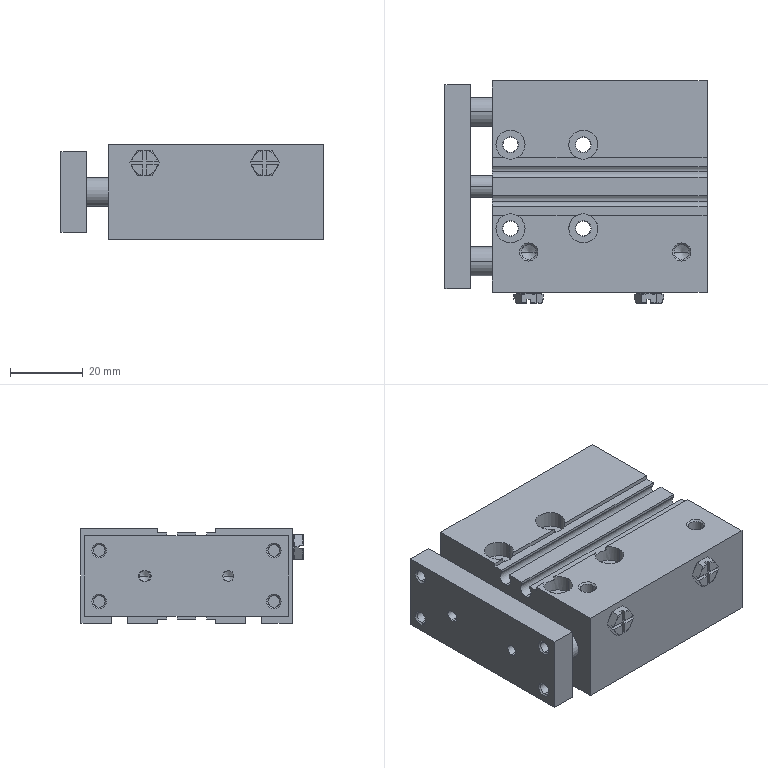Part | SolidWorks | 4 solids | 328 faces | box 72 x 61 x 26 mm | volume 82860 mm3 | plane 124 | cone 104 | cylinder 100 | commonest cylinder face diameters 3 x18 3.242 x16 4.134 x16 8 x16 4.3 x8 6 x8